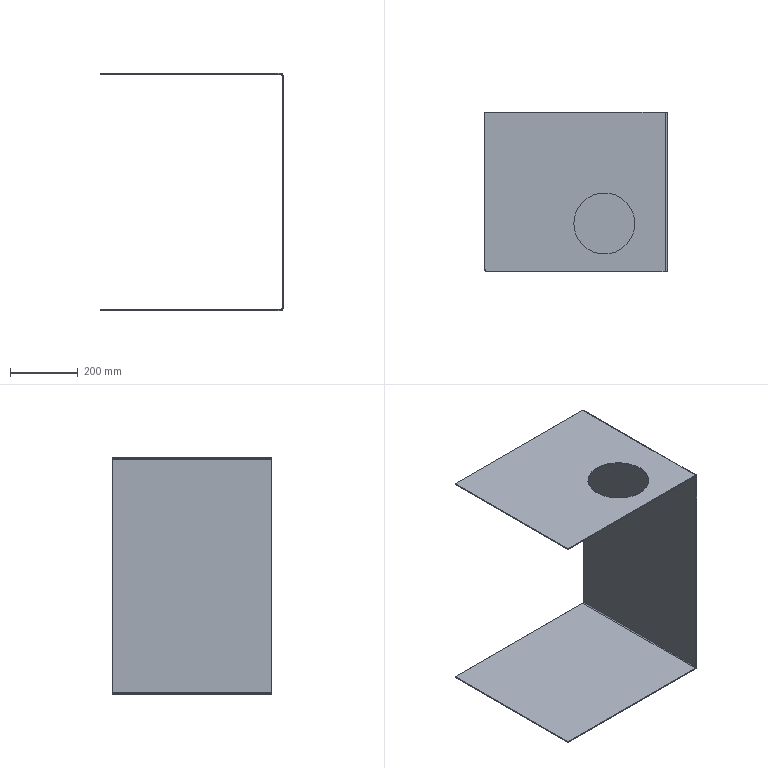Part | SolidWorks | features ICE 2, FlatPattern 1, SM3dBend 1, SMBaseFlange 1, SheetMetal 1 | 1 solid | 26 faces | box 537.004 x 469 x 699.997 mm | volume 2405774 mm3 | plane 18 | cylinder 8 | commonest cylinder face diameters 6 x2 10 x2 12 x2 180 x2
STEP:
#1=CARTESIAN_POINT('',(345.697,-287.133,696.997));
#2=VERTEX_POINT('',#1);
#3=CARTESIAN_POINT('',(165.697,-287.133,696.997));
#4=VERTEX_POINT('',#3);
#5=CARTESIAN_POINT('',(255.697,-287.133,696.997));
#6=DIRECTION('',(0.,0.,-1.));
#7=DIRECTION('',(-1.,0.,0.));
#8=AXIS2_PLACEMENT_3D('',#5,#6,#7);
#9=CIRCLE('',#8,90.);
#10=EDGE_CURVE('',#2,#4,#9,.T.);
#11=ORIENTED_EDGE('',*,*,#10,.F.);
#12=CARTESIAN_POINT('',(345.697,-287.133,693.997));
#13=VERTEX_POINT('',#12);
#14=CARTESIAN_POINT('',(345.697,-287.133,696.997));
#15=DIRECTION('',(0.,0.,-1.));
#16=VECTOR('',#15,1000.);
#17=LINE('',#14,#16);
#18=EDGE_CURVE('',#2,#13,#17,.T.);
#19=ORIENTED_EDGE('',*,*,#18,.T.);
#20=CARTESIAN_POINT('',(165.697,-287.133,693.997));
#21=VERTEX_POINT('',#20);
#22=CARTESIAN_POINT('',(255.697,-287.133,693.997));
#23=DIRECTION('',(0.,0.,-1.));
#24=DIRECTION('',(-1.,0.,0.));
#25=AXIS2_PLACEMENT_3D('',#22,#23,#24);
#26=CIRCLE('',#25,90.);
#27=EDGE_CURVE('',#13,#21,#26,.T.);
#28=ORIENTED_EDGE('',*,*,#27,.T.);
#29=CARTESIAN_POINT('',(165.697,-287.133,696.997));
#30=DIRECTION('',(0.,0.,-1.));
#31=VECTOR('',#30,1000.);
#32=LINE('',#29,#31);
#33=EDGE_CURVE('',#4,#21,#32,.T.);
#34=ORIENTED_EDGE('',*,*,#33,.F.);
#35=EDGE_LOOP('',(#11,#19,#28,#34));
#36=FACE_OUTER_BOUND('',#35,.T.);
#37=CARTESIAN_POINT('',(255.697,-287.133,696.997));
#38=DIRECTION('',(0.,0.,-1.));
#39=DIRECTION('',(-1.,0.,0.));
#40=AXIS2_PLACEMENT_3D('',#37,#38,#39);
#41=CYLINDRICAL_SURFACE('',#40,90.);
#42=ADVANCED_FACE('',(#36),#41,.F.);
#43=CARTESIAN_POINT('',(-96.307,40.867,-3.));
#44=VERTEX_POINT('',#43);
#45=CARTESIAN_POINT('',(-96.307,-423.133,-3.));
#46=VERTEX_POINT('',#45);
#47=CARTESIAN_POINT('',(-96.307,40.867,-3.));
#48=DIRECTION('',(0.,-1.,0.));
#49=VECTOR('',#48,1000.);
#50=LINE('',#47,#49);
#51=EDGE_CURVE('',#44,#46,#50,.T.);
#52=ORIENTED_EDGE('',*,*,#51,.T.);
#53=CARTESIAN_POINT('',(-96.307,-423.133,0.));
#54=VERTEX_POINT('',#53);
#55=CARTESIAN_POINT('',(-96.307,-423.133,0.));
#56=DIRECTION('',(0.,0.,-1.));
#57=VECTOR('',#56,1000.);
#58=LINE('',#55,#57);
#59=EDGE_CURVE('',#54,#46,#58,.T.);
#60=ORIENTED_EDGE('',*,*,#59,.F.);
#61=CARTESIAN_POINT('',(-96.307,40.867,0.));
#62=VERTEX_POINT('',#61);
#63=CARTESIAN_POINT('',(-96.307,40.867,0.));
#64=DIRECTION('',(0.,-1.,0.));
#65=VECTOR('',#64,1000.);
#66=LINE('',#63,#65);
#67=EDGE_CURVE('',#62,#54,#66,.T.);
#68=ORIENTED_EDGE('',*,*,#67,.F.);
#69=CARTESIAN_POINT('',(-96.307,40.867,-3.));
#70=DIRECTION('',(0.,0.,1.));
#71=VECTOR('',#70,1000.);
#72=LINE('',#69,#71);
#73=EDGE_CURVE('',#44,#62,#72,.T.);
#74=ORIENTED_EDGE('',*,*,#73,.F.);
#75=EDGE_LOOP('',(#52,#60,#68,#74));
#76=FACE_OUTER_BOUND('',#75,.T.);
#77=CARTESIAN_POINT('',(-96.307,40.867,-3.));
#78=DIRECTION('',(-1.,0.,0.));
#79=DIRECTION('',(0.,-1.,0.));
#80=AXIS2_PLACEMENT_3D('',#77,#78,#79);
#81=PLANE('',#80);
#82=ADVANCED_FACE('',(#76),#81,.T.);
#83=CARTESIAN_POINT('',(-91.307,-428.133,-3.));
#84=VERTEX_POINT('',#83);
#85=CARTESIAN_POINT('',(-91.307,-423.133,-3.));
#86=DIRECTION('',(0.,0.,1.));
#87=DIRECTION('',(1.,0.,0.));
#88=AXIS2_PLACEMENT_3D('',#85,#86,#87);
#89=CIRCLE('',#88,5.);
#90=EDGE_CURVE('',#46,#84,#89,.T.);
#91=ORIENTED_EDGE('',*,*,#90,.F.);
#92=ORIENTED_EDGE('',*,*,#51,.F.);
#93=CARTESIAN_POINT('',(434.697,40.867,-3.));
#94=VERTEX_POINT('',#93);
#95=CARTESIAN_POINT('',(-96.307,40.867,-3.));
#96=DIRECTION('',(-1.,0.,0.));
#97=VECTOR('',#96,1000.);
#98=LINE('',#95,#97);
#99=EDGE_CURVE('',#94,#44,#98,.T.);
#100=ORIENTED_EDGE('',*,*,#99,.F.);
#101=CARTESIAN_POINT('',(434.697,-428.133,-3.));
#102=VERTEX_POINT('',#101);
#103=CARTESIAN_POINT('',(434.697,0.,-3.));
#104=DIRECTION('',(0.,-1.,0.));
#105=VECTOR('',#104,1000.);
#106=LINE('',#103,#105);
#107=EDGE_CURVE('',#94,#102,#106,.T.);
#108=ORIENTED_EDGE('',*,*,#107,.T.);
#109=CARTESIAN_POINT('',(-96.307,-428.133,-3.));
#110=DIRECTION('',(1.,0.,0.));
#111=VECTOR('',#110,1000.);
#112=LINE('',#109,#111);
#113=EDGE_CURVE('',#84,#102,#112,.T.);
#114=ORIENTED_EDGE('',*,*,#113,.F.);
#115=EDGE_LOOP('',(#91,#92,#100,#108,#114));
#116=FACE_OUTER_BOUND('',#115,.T.);
#117=CARTESIAN_POINT('',(0.,0.,-3.));
#118=DIRECTION('',(0.,0.,1.));
#119=DIRECTION('',(1.,0.,0.));
#120=AXIS2_PLACEMENT_3D('',#117,#118,#119);
#121=PLANE('',#120);
#122=ADVANCED_FACE('',(#116),#121,.F.);
#123=ORIENTED_EDGE('',*,*,#67,.T.);
#124=CARTESIAN_POINT('',(-91.307,-428.133,0.));
#125=VERTEX_POINT('',#124);
#126=CARTESIAN_POINT('',(-91.307,-423.133,0.));
#127=DIRECTION('',(0.,0.,1.));
#128=DIRECTION('',(1.,0.,0.));
#129=AXIS2_PLACEMENT_3D('',#126,#127,#128);
#130=CIRCLE('',#129,5.);
#131=EDGE_CURVE('',#54,#125,#130,.T.);
#132=ORIENTED_EDGE('',*,*,#131,.T.);
#133=CARTESIAN_POINT('',(434.697,-428.133,0.));
#134=VERTEX_POINT('',#133);
#135=CARTESIAN_POINT('',(-96.307,-428.133,0.));
#136=DIRECTION('',(1.,0.,0.));
#137=VECTOR('',#136,1000.);
#138=LINE('',#135,#137);
#139=EDGE_CURVE('',#125,#134,#138,.T.);
#140=ORIENTED_EDGE('',*,*,#139,.T.);
#141=CARTESIAN_POINT('',(434.697,40.867,0.));
#142=VERTEX_POINT('',#141);
#143=CARTESIAN_POINT('',(434.697,0.,0.));
#144=DIRECTION('',(0.,-1.,0.));
#145=VECTOR('',#144,1000.);
#146=LINE('',#143,#145);
#147=EDGE_CURVE('',#142,#134,#146,.T.);
#148=ORIENTED_EDGE('',*,*,#147,.F.);
#149=CARTESIAN_POINT('',(-96.307,40.867,0.));
#150=DIRECTION('',(-1.,0.,0.));
#151=VECTOR('',#150,1000.);
#152=LINE('',#149,#151);
#153=EDGE_CURVE('',#142,#62,#152,.T.);
#154=ORIENTED_EDGE('',*,*,#153,.T.);
#155=EDGE_LOOP('',(#123,#132,#140,#148,#154));
#156=FACE_OUTER_BOUND('',#155,.T.);
#157=CARTESIAN_POINT('',(0.,0.,0.));
#158=DIRECTION('',(0.,0.,1.));
#159=DIRECTION('',(1.,0.,0.));
#160=AXIS2_PLACEMENT_3D('',#157,#158,#159);
#161=PLANE('',#160);
#162=ADVANCED_FACE('',(#156),#161,.T.);
#163=CARTESIAN_POINT('',(255.697,-287.133,696.997));
#164=DIRECTION('',(0.,0.,-1.));
#165=DIRECTION('',(-1.,0.,0.));
#166=AXIS2_PLACEMENT_3D('',#163,#164,#165);
#167=CIRCLE('',#166,90.);
#168=EDGE_CURVE('',#4,#2,#167,.T.);
#169=ORIENTED_EDGE('',*,*,#168,.T.);
#170=ORIENTED_EDGE('',*,*,#10,.T.);
#171=EDGE_LOOP('',(#169,#170));
#172=FACE_BOUND('',#171,.T.);
#173=CARTESIAN_POINT('',(-91.307,-428.133,696.997));
#174=VERTEX_POINT('',#173);
#175=CARTESIAN_POINT('',(-96.307,-423.133,696.997));
#176=VERTEX_POINT('',#175);
#177=CARTESIAN_POINT('',(-91.307,-423.133,696.997));
#178=DIRECTION('',(0.,0.,-1.));
#179=DIRECTION('',(-1.,0.,0.));
#180=AXIS2_PLACEMENT_3D('',#177,#178,#179);
#181=CIRCLE('',#180,5.);
#182=EDGE_CURVE('',#174,#176,#181,.T.);
#183=ORIENTED_EDGE('',*,*,#182,.F.);
#184=CARTESIAN_POINT('',(434.697,-428.133,696.997));
#185=VERTEX_POINT('',#184);
#186=CARTESIAN_POINT('',(1667.363,-428.133,696.997));
#187=DIRECTION('',(-1.,0.,0.));
#188=VECTOR('',#187,1000.);
#189=LINE('',#186,#188);
#190=EDGE_CURVE('',#185,#174,#189,.T.);
#191=ORIENTED_EDGE('',*,*,#190,.F.);
#192=CARTESIAN_POINT('',(434.697,40.867,696.997));
#193=VERTEX_POINT('',#192);
#194=CARTESIAN_POINT('',(434.697,0.,696.997));
#195=DIRECTION('',(0.,1.,0.));
#196=VECTOR('',#195,1000.);
#197=LINE('',#194,#196);
#198=EDGE_CURVE('',#185,#193,#197,.T.);
#199=ORIENTED_EDGE('',*,*,#198,.T.);
#200=CARTESIAN_POINT('',(-96.307,40.867,696.997));
#201=VERTEX_POINT('',#200);
#202=CARTESIAN_POINT('',(1667.363,40.867,696.997));
#203=DIRECTION('',(1.,0.,0.));
#204=VECTOR('',#203,1000.);
#205=LINE('',#202,#204);
#206=EDGE_CURVE('',#201,#193,#205,.T.);
#207=ORIENTED_EDGE('',*,*,#206,.F.);
#208=CARTESIAN_POINT('',(-96.307,40.867,696.997));
#209=DIRECTION('',(0.,1.,0.));
#210=VECTOR('',#209,1000.);
#211=LINE('',#208,#210);
#212=EDGE_CURVE('',#176,#201,#211,.T.);
#213=ORIENTED_EDGE('',*,*,#212,.F.);
#214=EDGE_LOOP('',(#183,#191,#199,#207,#213));
#215=FACE_OUTER_BOUND('',#214,.T.);
#216=CARTESIAN_POINT('',(1571.056,0.,696.997));
#217=DIRECTION('',(0.,0.,-1.));
#218=DIRECTION('',(-1.,0.,0.));
#219=AXIS2_PLACEMENT_3D('',#216,#217,#218);
#220=PLANE('',#219);
#221=ADVANCED_FACE('',(#172,#215),#220,.F.);
#222=CARTESIAN_POINT('',(255.697,-287.133,693.997));
#223=DIRECTION('',(0.,0.,-1.));
#224=DIRECTION('',(-1.,0.,0.));
#225=AXIS2_PLACEMENT_3D('',#222,#223,#224);
#226=CIRCLE('',#225,90.);
#227=EDGE_CURVE('',#21,#13,#226,.T.);
#228=ORIENTED_EDGE('',*,*,#227,.F.);
#229=ORIENTED_EDGE('',*,*,#27,.F.);
#230=EDGE_LOOP('',(#228,#229));
#231=FACE_BOUND('',#230,.T.);
#232=CARTESIAN_POINT('',(434.697,-428.133,693.997));
#233=VERTEX_POINT('',#232);
#234=CARTESIAN_POINT('',(-91.307,-428.133,693.997));
#235=VERTEX_POINT('',#234);
#236=CARTESIAN_POINT('',(1667.363,-428.133,693.997));
#237=DIRECTION('',(-1.,0.,0.));
#238=VECTOR('',#237,1000.);
#239=LINE('',#236,#238);
#240=EDGE_CURVE('',#233,#235,#239,.T.);
#241=ORIENTED_EDGE('',*,*,#240,.T.);
#242=CARTESIAN_POINT('',(-96.307,-423.133,693.997));
#243=VERTEX_POINT('',#242);
#244=CARTESIAN_POINT('',(-91.307,-423.133,693.997));
#245=DIRECTION('',(0.,0.,-1.));
#246=DIRECTION('',(-1.,0.,0.));
#247=AXIS2_PLACEMENT_3D('',#244,#245,#246);
#248=CIRCLE('',#247,5.);
#249=EDGE_CURVE('',#235,#243,#248,.T.);
#250=ORIENTED_EDGE('',*,*,#249,.T.);
#251=CARTESIAN_POINT('',(-96.307,40.867,693.997));
#252=VERTEX_POINT('',#251);
#253=CARTESIAN_POINT('',(-96.307,40.867,693.997));
#254=DIRECTION('',(0.,1.,0.));
#255=VECTOR('',#254,1000.);
#256=LINE('',#253,#255);
#257=EDGE_CURVE('',#243,#252,#256,.T.);
#258=ORIENTED_EDGE('',*,*,#257,.T.);
#259=CARTESIAN_POINT('',(434.697,40.867,693.997));
#260=VERTEX_POINT('',#259);
#261=CARTESIAN_POINT('',(1667.363,40.867,693.997));
#262=DIRECTION('',(1.,0.,0.));
#263=VECTOR('',#262,1000.);
#264=LINE('',#261,#263);
#265=EDGE_CURVE('',#252,#260,#264,.T.);
#266=ORIENTED_EDGE('',*,*,#265,.T.);
#267=CARTESIAN_POINT('',(434.697,0.,693.997));
#268=DIRECTION('',(0.,1.,0.));
#269=VECTOR('',#268,1000.);
#270=LINE('',#267,#269);
#271=EDGE_CURVE('',#233,#260,#270,.T.);
#272=ORIENTED_EDGE('',*,*,#271,.F.);
#273=EDGE_LOOP('',(#241,#250,#258,#266,#272));
#274=FACE_OUTER_BOUND('',#273,.T.);
#275=CARTESIAN_POINT('',(1571.056,0.,693.997));
#276=DIRECTION('',(0.,0.,-1.));
#277=DIRECTION('',(-1.,0.,0.));
#278=AXIS2_PLACEMENT_3D('',#275,#276,#277);
#279=PLANE('',#278);
#280=ADVANCED_FACE('',(#231,#274),#279,.T.);
#281=ORIENTED_EDGE('',*,*,#190,.T.);
#282=CARTESIAN_POINT('',(-91.307,-428.133,693.997));
#283=DIRECTION('',(0.,0.,1.));
#284=VECTOR('',#283,1000.);
#285=LINE('',#282,#284);
#286=EDGE_CURVE('',#235,#174,#285,.T.);
#287=ORIENTED_EDGE('',*,*,#286,.F.);
#288=ORIENTED_EDGE('',*,*,#240,.F.);
#289=CARTESIAN_POINT('',(434.697,-428.133,696.997));
#290=DIRECTION('',(0.,0.,-1.));
#291=VECTOR('',#290,1000.);
#292=LINE('',#289,#291);
#293=EDGE_CURVE('',#185,#233,#292,.T.);
#294=ORIENTED_EDGE('',*,*,#293,.F.);
#295=EDGE_LOOP('',(#281,#287,#288,#294));
#296=FACE_OUTER_BOUND('',#295,.T.);
#297=CARTESIAN_POINT('',(1667.363,-428.133,696.997));
#298=DIRECTION('',(0.,-1.,0.));
#299=DIRECTION('',(0.,0.,1.));
#300=AXIS2_PLACEMENT_3D('',#297,#298,#299);
#301=PLANE('',#300);
#302=ADVANCED_FACE('',(#296),#301,.T.);
#303=CARTESIAN_POINT('',(437.697,40.867,690.997));
#304=VERTEX_POINT('',#303);
#305=CARTESIAN_POINT('',(437.697,40.867,3.));
#306=VERTEX_POINT('',#305);
#307=CARTESIAN_POINT('',(437.697,40.867,-534.836));
#308=DIRECTION('',(0.,0.,-1.));
#309=VECTOR('',#308,1000.);
#310=LINE('',#307,#309);
#311=EDGE_CURVE('',#304,#306,#310,.T.);
#312=ORIENTED_EDGE('',*,*,#311,.F.);
#313=CARTESIAN_POINT('',(440.697,40.867,690.997));
#314=VERTEX_POINT('',#313);
#315=CARTESIAN_POINT('',(440.697,40.867,690.997));
#316=DIRECTION('',(1.,0.,0.));
#317=VECTOR('',#316,1000.);
#318=LINE('',#315,#317);
#319=EDGE_CURVE('',#304,#314,#318,.T.);
#320=ORIENTED_EDGE('',*,*,#319,.T.);
#321=CARTESIAN_POINT('',(440.697,40.867,3.));
#322=VERTEX_POINT('',#321);
#323=CARTESIAN_POINT('',(440.697,40.867,-534.836));
#324=DIRECTION('',(0.,0.,-1.));
#325=VECTOR('',#324,1000.);
#326=LINE('',#323,#325);
#327=EDGE_CURVE('',#314,#322,#326,.T.);
#328=ORIENTED_EDGE('',*,*,#327,.T.);
#329=CARTESIAN_POINT('',(440.697,40.867,3.));
#330=DIRECTION('',(-1.,0.,0.));
#331=VECTOR('',#330,1000.);
#332=LINE('',#329,#331);
#333=EDGE_CURVE('',#322,#306,#332,.T.);
#334=ORIENTED_EDGE('',*,*,#333,.T.);
#335=EDGE_LOOP('',(#312,#320,#328,#334));
#336=FACE_OUTER_BOUND('',#335,.T.);
#337=CARTESIAN_POINT('',(440.697,40.867,-534.836));
#338=DIRECTION('',(0.,1.,0.));
#339=DIRECTION('',(-1.,0.,0.));
#340=AXIS2_PLACEMENT_3D('',#337,#338,#339);
#341=PLANE('',#340);
#342=ADVANCED_FACE('',(#336),#341,.T.);
#343=CARTESIAN_POINT('',(440.697,-428.133,3.));
#344=VERTEX_POINT('',#343);
#345=CARTESIAN_POINT('',(440.697,-428.133,690.997));
#346=VERTEX_POINT('',#345);
#347=CARTESIAN_POINT('',(440.697,-428.133,-534.836));
#348=DIRECTION('',(0.,0.,1.));
#349=VECTOR('',#348,1000.);
#350=LINE('',#347,#349);
#351=EDGE_CURVE('',#344,#346,#350,.T.);
#352=ORIENTED_EDGE('',*,*,#351,.T.);
#353=CARTESIAN_POINT('',(437.697,-428.133,690.997));
#354=VERTEX_POINT('',#353);
#355=CARTESIAN_POINT('',(440.697,-428.133,690.997));
#356=DIRECTION('',(-1.,0.,0.));
#357=VECTOR('',#356,1000.);
#358=LINE('',#355,#357);
#359=EDGE_CURVE('',#346,#354,#358,.T.);
#360=ORIENTED_EDGE('',*,*,#359,.T.);
#361=CARTESIAN_POINT('',(437.697,-428.133,3.));
#362=VERTEX_POINT('',#361);
#363=CARTESIAN_POINT('',(437.697,-428.133,-534.836));
#364=DIRECTION('',(0.,0.,1.));
#365=VECTOR('',#364,1000.);
#366=LINE('',#363,#365);
#367=EDGE_CURVE('',#362,#354,#366,.T.);
#368=ORIENTED_EDGE('',*,*,#367,.F.);
#369=CARTESIAN_POINT('',(440.697,-428.133,3.));
#370=DIRECTION('',(1.,0.,0.));
#371=VECTOR('',#370,1000.);
#372=LINE('',#369,#371);
#373=EDGE_CURVE('',#362,#344,#372,.T.);
#374=ORIENTED_EDGE('',*,*,#373,.T.);
#375=EDGE_LOOP('',(#352,#360,#368,#374));
#376=FACE_OUTER_BOUND('',#375,.T.);
#377=CARTESIAN_POINT('',(440.697,-428.133,-534.836));
#378=DIRECTION('',(0.,-1.,0.));
#379=DIRECTION('',(1.,0.,0.));
#380=AXIS2_PLACEMENT_3D('',#377,#378,#379);
#381=PLANE('',#380);
#382=ADVANCED_FACE('',(#376),#381,.T.);
#383=ORIENTED_EDGE('',*,*,#367,.T.);
#384=CARTESIAN_POINT('',(437.697,0.,690.997));
#385=DIRECTION('',(0.,1.,0.));
#386=VECTOR('',#385,1000.);
#387=LINE('',#384,#386);
#388=EDGE_CURVE('',#354,#304,#387,.T.);
#389=ORIENTED_EDGE('',*,*,#388,.T.);
#390=ORIENTED_EDGE('',*,*,#311,.T.);
#391=CARTESIAN_POINT('',(437.697,0.,3.));
#392=DIRECTION('',(0.,-1.,0.));
#393=VECTOR('',#392,1000.);
#394=LINE('',#391,#393);
#395=EDGE_CURVE('',#306,#362,#394,.T.);
#396=ORIENTED_EDGE('',*,*,#395,.T.);
#397=EDGE_LOOP('',(#383,#389,#390,#396));
#398=FACE_OUTER_BOUND('',#397,.T.);
#399=CARTESIAN_POINT('',(437.697,0.,-438.53));
#400=DIRECTION('',(-1.,0.,0.));
#401=DIRECTION('',(0.,0.,1.));
#402=AXIS2_PLACEMENT_3D('',#399,#400,#401);
#403=PLANE('',#402);
#404=ADVANCED_FACE('',(#398),#403,.T.);
#405=CARTESIAN_POINT('',(440.697,0.,690.997));
#406=DIRECTION('',(0.,1.,0.));
#407=VECTOR('',#406,1000.);
#408=LINE('',#405,#407);
#409=EDGE_CURVE('',#346,#314,#408,.T.);
#410=ORIENTED_EDGE('',*,*,#409,.F.);
#411=ORIENTED_EDGE('',*,*,#351,.F.);
#412=CARTESIAN_POINT('',(440.697,0.,3.));
#413=DIRECTION('',(0.,-1.,0.));
#414=VECTOR('',#413,1000.);
#415=LINE('',#412,#414);
#416=EDGE_CURVE('',#322,#344,#415,.T.);
#417=ORIENTED_EDGE('',*,*,#416,.F.);
#418=ORIENTED_EDGE('',*,*,#327,.F.);
#419=EDGE_LOOP('',(#410,#411,#417,#418));
#420=FACE_OUTER_BOUND('',#419,.T.);
#421=CARTESIAN_POINT('',(440.697,0.,-438.53));
#422=DIRECTION('',(-1.,0.,0.));
#423=DIRECTION('',(0.,0.,1.));
#424=AXIS2_PLACEMENT_3D('',#421,#422,#423);
#425=PLANE('',#424);
#426=ADVANCED_FACE('',(#420),#425,.F.);
#427=CARTESIAN_POINT('',(-91.307,-428.133,0.));
#428=DIRECTION('',(0.,0.,-1.));
#429=VECTOR('',#428,1000.);
#430=LINE('',#427,#429);
#431=EDGE_CURVE('',#125,#84,#430,.T.);
#432=ORIENTED_EDGE('',*,*,#431,.T.);
#433=ORIENTED_EDGE('',*,*,#113,.T.);
#434=CARTESIAN_POINT('',(434.697,-428.133,-3.));
#435=DIRECTION('',(0.,0.,-1.));
#436=VECTOR('',#435,1000.);
#437=LINE('',#434,#436);
#438=EDGE_CURVE('',#134,#102,#437,.T.);
#439=ORIENTED_EDGE('',*,*,#438,.F.);
#440=ORIENTED_EDGE('',*,*,#139,.F.);
#441=EDGE_LOOP('',(#432,#433,#439,#440));
#442=FACE_OUTER_BOUND('',#441,.T.);
#443=CARTESIAN_POINT('',(-96.307,-428.133,-3.));
#444=DIRECTION('',(0.,-1.,0.));
#445=DIRECTION('',(0.,0.,-1.));
#446=AXIS2_PLACEMENT_3D('',#443,#444,#445);
#447=PLANE('',#446);
#448=ADVANCED_FACE('',(#442),#447,.T.);
#449=CARTESIAN_POINT('',(434.697,40.867,-3.));
#450=DIRECTION('',(0.,0.,1.));
#451=VECTOR('',#450,1000.);
#452=LINE('',#449,#451);
#453=EDGE_CURVE('',#94,#142,#452,.T.);
#454=ORIENTED_EDGE('',*,*,#453,.F.);
#455=ORIENTED_EDGE('',*,*,#99,.T.);
#456=ORIENTED_EDGE('',*,*,#73,.T.);
#457=ORIENTED_EDGE('',*,*,#153,.F.);
#458=EDGE_LOOP('',(#454,#455,#456,#457));
#459=FACE_OUTER_BOUND('',#458,.T.);
#460=CARTESIAN_POINT('',(-96.307,40.867,-3.));
#461=DIRECTION('',(0.,1.,0.));
#462=DIRECTION('',(0.,0.,1.));
#463=AXIS2_PLACEMENT_3D('',#460,#461,#462);
#464=PLANE('',#463);
#465=ADVANCED_FACE('',(#459),#464,.T.);
#466=ORIENTED_EDGE('',*,*,#453,.T.);
#467=CARTESIAN_POINT('',(434.697,40.867,3.));
#468=DIRECTION('',(0.,-1.,0.));
#469=DIRECTION('',(1.,0.,0.));
#470=AXIS2_PLACEMENT_3D('',#467,#468,#469);
#471=CIRCLE('',#470,3.);
#472=EDGE_CURVE('',#142,#306,#471,.T.);
#473=ORIENTED_EDGE('',*,*,#472,.T.);
#474=ORIENTED_EDGE('',*,*,#333,.F.);
#475=CARTESIAN_POINT('',(434.697,40.867,3.));
#476=DIRECTION('',(0.,-1.,0.));
#477=DIRECTION('',(0.,0.,1.));
#478=AXIS2_PLACEMENT_3D('',#475,#476,#477);
#479=CIRCLE('',#478,6.);
#480=EDGE_CURVE('',#94,#322,#479,.T.);
#481=ORIENTED_EDGE('',*,*,#480,.F.);
#482=EDGE_LOOP('',(#466,#473,#474,#481));
#483=FACE_OUTER_BOUND('',#482,.T.);
#484=CARTESIAN_POINT('',(434.697,40.867,3.));
#485=DIRECTION('',(0.,1.,0.));
#486=DIRECTION('',(0.,0.,1.));
#487=AXIS2_PLACEMENT_3D('',#484,#485,#486);
#488=PLANE('',#487);
#489=ADVANCED_FACE('',(#483),#488,.T.);
#490=ORIENTED_EDGE('',*,*,#373,.F.);
#491=CARTESIAN_POINT('',(434.697,-428.133,3.));
#492=DIRECTION('',(0.,1.,0.));
#493=DIRECTION('',(1.,0.,0.));
#494=AXIS2_PLACEMENT_3D('',#491,#492,#493);
#495=CIRCLE('',#494,3.);
#496=EDGE_CURVE('',#362,#134,#495,.T.);
#497=ORIENTED_EDGE('',*,*,#496,.T.);
#498=ORIENTED_EDGE('',*,*,#438,.T.);
#499=CARTESIAN_POINT('',(434.697,-428.133,3.));
#500=DIRECTION('',(0.,1.,0.));
#501=DIRECTION('',(0.,0.,-1.));
#502=AXIS2_PLACEMENT_3D('',#499,#500,#501);
#503=CIRCLE('',#502,6.);
#504=EDGE_CURVE('',#344,#102,#503,.T.);
#505=ORIENTED_EDGE('',*,*,#504,.F.);
#506=EDGE_LOOP('',(#490,#497,#498,#505));
#507=FACE_OUTER_BOUND('',#506,.T.);
#508=CARTESIAN_POINT('',(434.697,-428.133,3.));
#509=DIRECTION('',(0.,-1.,0.));
#510=DIRECTION('',(0.,0.,-1.));
#511=AXIS2_PLACEMENT_3D('',#508,#509,#510);
#512=PLANE('',#511);
#513=ADVANCED_FACE('',(#507),#512,.T.);
#514=ORIENTED_EDGE('',*,*,#504,.T.);
#515=ORIENTED_EDGE('',*,*,#107,.F.);
#516=ORIENTED_EDGE('',*,*,#480,.T.);
#517=ORIENTED_EDGE('',*,*,#416,.T.);
#518=EDGE_LOOP('',(#514,#515,#516,#517));
#519=FACE_OUTER_BOUND('',#518,.T.);
#520=CARTESIAN_POINT('',(434.697,275.426,3.));
#521=DIRECTION('',(0.,-1.,0.));
#522=DIRECTION('',(1.,0.,0.));
#523=AXIS2_PLACEMENT_3D('',#520,#521,#522);
#524=CYLINDRICAL_SURFACE('',#523,6.);
#525=ADVANCED_FACE('',(#519),#524,.T.);
#526=ORIENTED_EDGE('',*,*,#496,.F.);
#527=ORIENTED_EDGE('',*,*,#395,.F.);
#528=ORIENTED_EDGE('',*,*,#472,.F.);
#529=ORIENTED_EDGE('',*,*,#147,.T.);
#530=EDGE_LOOP('',(#526,#527,#528,#529));
#531=FACE_OUTER_BOUND('',#530,.T.);
#532=CARTESIAN_POINT('',(434.697,275.426,3.));
#533=DIRECTION('',(0.,-1.,0.));
#534=DIRECTION('',(1.,0.,0.));
#535=AXIS2_PLACEMENT_3D('',#532,#533,#534);
#536=CYLINDRICAL_SURFACE('',#535,3.);
#537=ADVANCED_FACE('',(#531),#536,.F.);
#538=ORIENTED_EDGE('',*,*,#293,.T.);
#539=CARTESIAN_POINT('',(434.697,-428.133,690.997));
#540=DIRECTION('',(0.,1.,0.));
#541=DIRECTION('',(1.,0.,0.));
#542=AXIS2_PLACEMENT_3D('',#539,#540,#541);
#543=CIRCLE('',#542,3.);
#544=EDGE_CURVE('',#233,#354,#543,.T.);
#545=ORIENTED_EDGE('',*,*,#544,.T.);
#546=ORIENTED_EDGE('',*,*,#359,.F.);
#547=CARTESIAN_POINT('',(434.697,-428.133,690.997));
#548=DIRECTION('',(0.,1.,0.));
#549=DIRECTION('',(0.,0.,-1.));
#550=AXIS2_PLACEMENT_3D('',#547,#548,#549);
#551=CIRCLE('',#550,6.);
#552=EDGE_CURVE('',#185,#346,#551,.T.);
#553=ORIENTED_EDGE('',*,*,#552,.F.);
#554=EDGE_LOOP('',(#538,#545,#546,#553));
#555=FACE_OUTER_BOUND('',#554,.T.);
#556=CARTESIAN_POINT('',(434.697,-428.133,690.997));
#557=DIRECTION('',(0.,-1.,0.));
#558=DIRECTION('',(0.,0.,-1.));
#559=AXIS2_PLACEMENT_3D('',#556,#557,#558);
#560=PLANE('',#559);
#561=ADVANCED_FACE('',(#555),#560,.T.);
#562=ORIENTED_EDGE('',*,*,#319,.F.);
#563=CARTESIAN_POINT('',(434.697,40.867,690.997));
#564=DIRECTION('',(0.,-1.,0.));
#565=DIRECTION('',(1.,0.,0.));
#566=AXIS2_PLACEMENT_3D('',#563,#564,#565);
#567=CIRCLE('',#566,3.);
#568=EDGE_CURVE('',#304,#260,#567,.T.);
#569=ORIENTED_EDGE('',*,*,#568,.T.);
#570=CARTESIAN_POINT('',(434.697,40.867,696.997));
#571=DIRECTION('',(0.,0.,1.));
#572=VECTOR('',#571,1000.);
#573=LINE('',#570,#572);
#574=EDGE_CURVE('',#260,#193,#573,.T.);
#575=ORIENTED_EDGE('',*,*,#574,.T.);
#576=CARTESIAN_POINT('',(434.697,40.867,690.997));
#577=DIRECTION('',(0.,-1.,0.));
#578=DIRECTION('',(0.,0.,1.));
#579=AXIS2_PLACEMENT_3D('',#576,#577,#578);
#580=CIRCLE('',#579,6.);
#581=EDGE_CURVE('',#314,#193,#580,.T.);
#582=ORIENTED_EDGE('',*,*,#581,.F.);
#583=EDGE_LOOP('',(#562,#569,#575,#582));
#584=FACE_OUTER_BOUND('',#583,.T.);
#585=CARTESIAN_POINT('',(434.697,40.867,690.997));
#586=DIRECTION('',(0.,1.,0.));
#587=DIRECTION('',(0.,0.,1.));
#588=AXIS2_PLACEMENT_3D('',#585,#586,#587);
#589=PLANE('',#588);
#590=ADVANCED_FACE('',(#584),#589,.T.);
#591=ORIENTED_EDGE('',*,*,#581,.T.);
#592=ORIENTED_EDGE('',*,*,#198,.F.);
#593=ORIENTED_EDGE('',*,*,#552,.T.);
#594=ORIENTED_EDGE('',*,*,#409,.T.);
#595=EDGE_LOOP('',(#591,#592,#593,#594));
#596=FACE_OUTER_BOUND('',#595,.T.);
#597=CARTESIAN_POINT('',(434.697,275.426,690.997));
#598=DIRECTION('',(0.,-1.,0.));
#599=DIRECTION('',(1.,0.,0.));
#600=AXIS2_PLACEMENT_3D('',#597,#598,#599);
#601=CYLINDRICAL_SURFACE('',#600,6.);
#602=ADVANCED_FACE('',(#596),#601,.T.);
#603=ORIENTED_EDGE('',*,*,#568,.F.);
#604=ORIENTED_EDGE('',*,*,#388,.F.);
#605=ORIENTED_EDGE('',*,*,#544,.F.);
#606=ORIENTED_EDGE('',*,*,#271,.T.);
#607=EDGE_LOOP('',(#603,#604,#605,#606));
#608=FACE_OUTER_BOUND('',#607,.T.);
#609=CARTESIAN_POINT('',(434.697,275.426,690.997));
#610=DIRECTION('',(0.,-1.,0.));
#611=DIRECTION('',(1.,0.,0.));
#612=AXIS2_PLACEMENT_3D('',#609,#610,#611);
#613=CYLINDRICAL_SURFACE('',#612,3.);
#614=ADVANCED_FACE('',(#608),#613,.F.);
#615=CARTESIAN_POINT('',(-96.307,-423.133,693.997));
#616=DIRECTION('',(0.,0.,1.));
#617=VECTOR('',#616,1000.);
#618=LINE('',#615,#617);
#619=EDGE_CURVE('',#243,#176,#618,.T.);
#620=ORIENTED_EDGE('',*,*,#619,.T.);
#621=ORIENTED_EDGE('',*,*,#212,.T.);
#622=CARTESIAN_POINT('',(-96.307,40.867,696.997));
#623=DIRECTION('',(0.,0.,-1.));
#624=VECTOR('',#623,1000.);
#625=LINE('',#622,#624);
#626=EDGE_CURVE('',#201,#252,#625,.T.);
#627=ORIENTED_EDGE('',*,*,#626,.T.);
#628=ORIENTED_EDGE('',*,*,#257,.F.);
#629=EDGE_LOOP('',(#620,#621,#627,#628));
#630=FACE_OUTER_BOUND('',#629,.T.);
#631=CARTESIAN_POINT('',(-96.307,40.867,696.997));
#632=DIRECTION('',(-1.,0.,0.));
#633=DIRECTION('',(0.,0.,1.));
#634=AXIS2_PLACEMENT_3D('',#631,#632,#633);
#635=PLANE('',#634);
#636=ADVANCED_FACE('',(#630),#635,.T.);
#637=ORIENTED_EDGE('',*,*,#574,.F.);
#638=ORIENTED_EDGE('',*,*,#265,.F.);
#639=ORIENTED_EDGE('',*,*,#626,.F.);
#640=ORIENTED_EDGE('',*,*,#206,.T.);
#641=EDGE_LOOP('',(#637,#638,#639,#640));
#642=FACE_OUTER_BOUND('',#641,.T.);
#643=CARTESIAN_POINT('',(1667.363,40.867,696.997));
#644=DIRECTION('',(0.,1.,0.));
#645=DIRECTION('',(0.,0.,-1.));
#646=AXIS2_PLACEMENT_3D('',#643,#644,#645);
#647=PLANE('',#646);
#648=ADVANCED_FACE('',(#642),#647,.T.);
#649=ORIENTED_EDGE('',*,*,#18,.F.);
#650=ORIENTED_EDGE('',*,*,#168,.F.);
#651=ORIENTED_EDGE('',*,*,#33,.T.);
#652=ORIENTED_EDGE('',*,*,#227,.T.);
#653=EDGE_LOOP('',(#649,#650,#651,#652));
#654=FACE_OUTER_BOUND('',#653,.T.);
#655=CARTESIAN_POINT('',(255.697,-287.133,696.997));
#656=DIRECTION('',(0.,0.,-1.));
#657=DIRECTION('',(-1.,0.,0.));
#658=AXIS2_PLACEMENT_3D('',#655,#656,#657);
#659=CYLINDRICAL_SURFACE('',#658,90.);
#660=ADVANCED_FACE('',(#654),#659,.F.);
#661=ORIENTED_EDGE('',*,*,#619,.F.);
#662=ORIENTED_EDGE('',*,*,#249,.F.);
#663=ORIENTED_EDGE('',*,*,#286,.T.);
#664=ORIENTED_EDGE('',*,*,#182,.T.);
#665=EDGE_LOOP('',(#661,#662,#663,#664));
#666=FACE_OUTER_BOUND('',#665,.T.);
#667=CARTESIAN_POINT('',(-91.307,-423.133,693.997));
#668=DIRECTION('',(0.,0.,-1.));
#669=DIRECTION('',(-1.,0.,0.));
#670=AXIS2_PLACEMENT_3D('',#667,#668,#669);
#671=CYLINDRICAL_SURFACE('',#670,5.);
#672=ADVANCED_FACE('',(#666),#671,.T.);
#673=ORIENTED_EDGE('',*,*,#431,.F.);
#674=ORIENTED_EDGE('',*,*,#131,.F.);
#675=ORIENTED_EDGE('',*,*,#59,.T.);
#676=ORIENTED_EDGE('',*,*,#90,.T.);
#677=EDGE_LOOP('',(#673,#674,#675,#676));
#678=FACE_OUTER_BOUND('',#677,.T.);
#679=CARTESIAN_POINT('',(-91.307,-423.133,0.));
#680=DIRECTION('',(0.,0.,1.));
#681=DIRECTION('',(1.,0.,0.));
#682=AXIS2_PLACEMENT_3D('',#679,#680,#681);
#683=CYLINDRICAL_SURFACE('',#682,5.);
#684=ADVANCED_FACE('',(#678),#683,.T.);
#685=CLOSED_SHELL('',(#42,#82,#122,#162,#221,#280,#302,#342,#382,#404,#426,#448,#465,#489,#513,#525,#537,#561,#590,#602,#614,#636,#648,#660,#672,#684));
#686=MANIFOLD_SOLID_BREP('',#685);
#687=CARTESIAN_POINT('',(0.,0.,0.));
#688=DIRECTION('',(0.,0.,1.));
#689=DIRECTION('',(1.,0.,0.));
#690=AXIS2_PLACEMENT_3D('',#687,#688,#689);
#691=(LENGTH_UNIT()NAMED_UNIT(*)SI_UNIT(.MILLI.,.METRE.));
#692=UNCERTAINTY_MEASURE_WITH_UNIT(LENGTH_MEASURE(0.00001),#691,'','');
#693=(NAMED_UNIT(*)PLANE_ANGLE_UNIT()SI_UNIT($,.RADIAN.));
#694=(NAMED_UNIT(*)SI_UNIT($,.STERADIAN.)SOLID_ANGLE_UNIT());
#695=(GEOMETRIC_REPRESENTATION_CONTEXT(3)GLOBAL_UNCERTAINTY_ASSIGNED_CONTEXT((#692))GLOBAL_UNIT_ASSIGNED_CONTEXT((#691,#693,#694))REPRESENTATION_CONTEXT('',''));
#696=ADVANCED_BREP_SHAPE_REPRESENTATION('',(#686,#690),#695);